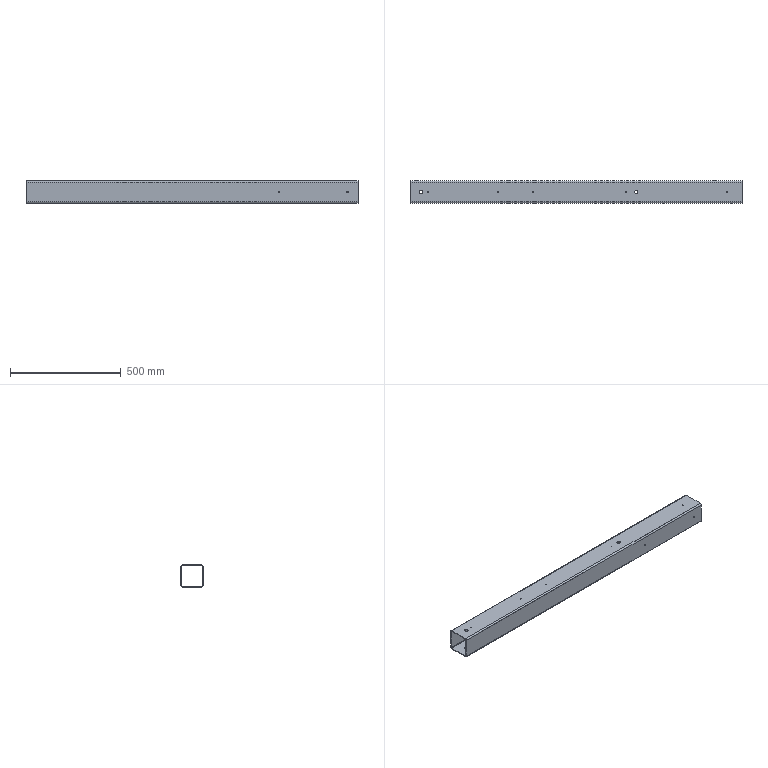Part | STEP file | [03] | 1 solid | 44 faces | box 1497 x 100 x 100 mm | volume 1811999 mm3 | cylinder 34 | plane 10 | commonest cylinder face diameters 4 x10 15 x8 6 x4 6.4 x4 12 x4 12.8 x4